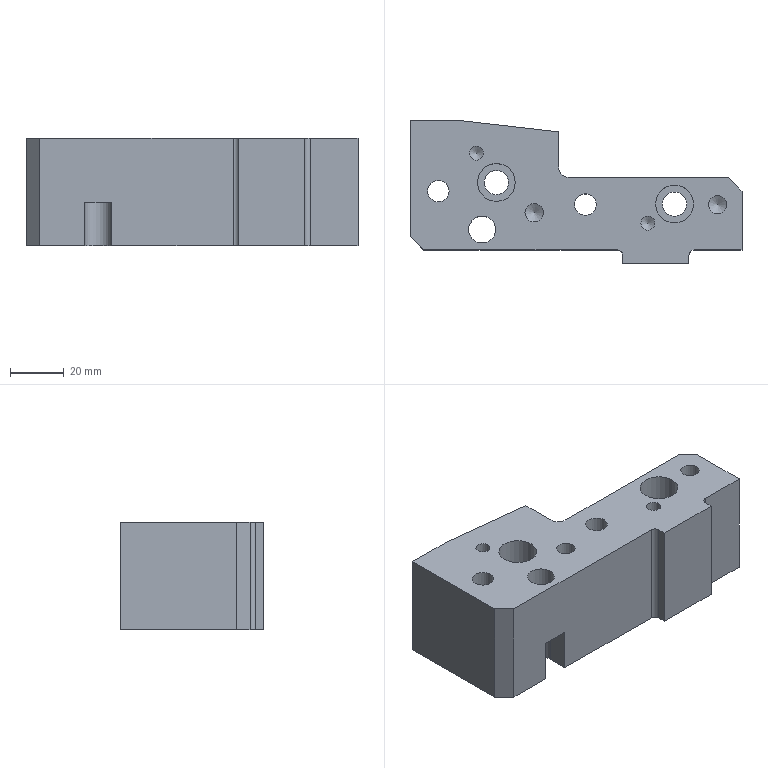Part | STEP file | gslz 2016.10.28-13_id1530_x_t | 1 solid | 38 faces | box 123 x 53 x 40 mm | volume 161709 mm3 | plane 19 | cylinder 14 | cone 4 | other 1 | commonest cylinder face diameters 8 x3 4 x2 5.2 x2 6.8 x2 9 x2 14 x2